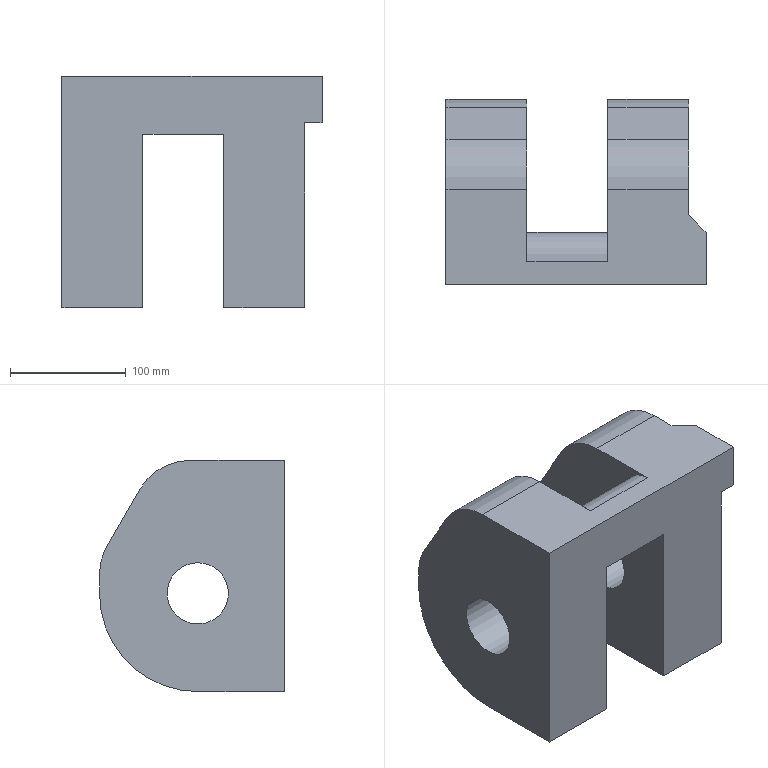Part | NX | features solid 2 | 1 solid | 25 faces | box 225 x 160 x 200 mm | volume 3809518 mm3 | plane 16 | cylinder 9 | commonest cylinder face diameters 100 x4 53 x2 170 x2 50 x1
STEP:
#1=CARTESIAN_POINT('',(925.,625.,111.5));
#2=VERTEX_POINT('',#1);
#3=CARTESIAN_POINT('',(925.,625.,85.));
#4=DIRECTION('',(-1.,0.,0.));
#5=DIRECTION('',(0.,0.,1.));
#6=AXIS2_PLACEMENT_3D('',#3,#4,#5);
#7=CIRCLE('',#6,26.5);
#8=EDGE_CURVE('',#2,#2,#7,.T.);
#9=ORIENTED_EDGE('',*,*,#8,.T.);
#10=EDGE_LOOP('',(#9));
#11=FACE_BOUND('',#10,.T.);
#12=CARTESIAN_POINT('',(995.,625.,111.5));
#13=VERTEX_POINT('',#12);
#14=CARTESIAN_POINT('',(995.,625.,85.));
#15=DIRECTION('',(-1.,0.,0.));
#16=DIRECTION('',(0.,0.,1.));
#17=AXIS2_PLACEMENT_3D('',#14,#15,#16);
#18=CIRCLE('',#17,26.5);
#19=EDGE_CURVE('',#13,#13,#18,.T.);
#20=ORIENTED_EDGE('',*,*,#19,.F.);
#21=EDGE_LOOP('',(#20));
#22=FACE_BOUND('',#21,.T.);
#23=CARTESIAN_POINT('',(915.,625.,85.));
#24=DIRECTION('',(1.,0.,0.));
#25=DIRECTION('',(0.,0.,1.));
#26=AXIS2_PLACEMENT_3D('',#23,#24,#25);
#27=CYLINDRICAL_SURFACE('',#26,26.5);
#28=ADVANCED_FACE('',(#11,#22),#27,.F.);
#29=CARTESIAN_POINT('',(995.,631.906,200.));
#30=VERTEX_POINT('',#29);
#31=CARTESIAN_POINT('',(995.,675.207,175.));
#32=VERTEX_POINT('',#31);
#33=CARTESIAN_POINT('',(995.,631.906,150.));
#34=DIRECTION('',(-1.,0.,0.));
#35=DIRECTION('',(0.,0.,1.));
#36=AXIS2_PLACEMENT_3D('',#33,#34,#35);
#37=CIRCLE('',#36,50.);
#38=EDGE_CURVE('',#30,#32,#37,.T.);
#39=ORIENTED_EDGE('',*,*,#38,.T.);
#40=CARTESIAN_POINT('',(925.,675.207,175.));
#41=VERTEX_POINT('',#40);
#42=CARTESIAN_POINT('',(915.,675.207,175.));
#43=DIRECTION('',(1.,0.,0.));
#44=VECTOR('',#43,1000.);
#45=LINE('',#42,#44);
#46=EDGE_CURVE('',#41,#32,#45,.T.);
#47=ORIENTED_EDGE('',*,*,#46,.F.);
#48=CARTESIAN_POINT('',(925.,631.906,200.));
#49=VERTEX_POINT('',#48);
#50=CARTESIAN_POINT('',(925.,631.906,150.));
#51=DIRECTION('',(-1.,0.,0.));
#52=DIRECTION('',(0.,0.,1.));
#53=AXIS2_PLACEMENT_3D('',#50,#51,#52);
#54=CIRCLE('',#53,50.);
#55=EDGE_CURVE('',#49,#41,#54,.T.);
#56=ORIENTED_EDGE('',*,*,#55,.F.);
#57=CARTESIAN_POINT('',(915.,631.906,200.));
#58=DIRECTION('',(1.,0.,0.));
#59=VECTOR('',#58,1000.);
#60=LINE('',#57,#59);
#61=EDGE_CURVE('',#49,#30,#60,.T.);
#62=ORIENTED_EDGE('',*,*,#61,.T.);
#63=EDGE_LOOP('',(#39,#47,#56,#62));
#64=FACE_BOUND('',#63,.T.);
#65=CARTESIAN_POINT('',(915.,631.906,150.));
#66=DIRECTION('',(1.,0.,0.));
#67=DIRECTION('',(0.,0.,1.));
#68=AXIS2_PLACEMENT_3D('',#65,#66,#67);
#69=CYLINDRICAL_SURFACE('',#68,50.);
#70=ADVANCED_FACE('',(#64),#69,.T.);
#71=CARTESIAN_POINT('',(995.,703.301,126.34));
#72=VERTEX_POINT('',#71);
#73=CARTESIAN_POINT('',(995.,655.,210.));
#74=DIRECTION('',(0.,0.5,-0.866));
#75=VECTOR('',#74,1000.);
#76=LINE('',#73,#75);
#77=EDGE_CURVE('',#32,#72,#76,.T.);
#78=ORIENTED_EDGE('',*,*,#77,.T.);
#79=CARTESIAN_POINT('',(925.,703.301,126.34));
#80=VERTEX_POINT('',#79);
#81=CARTESIAN_POINT('',(915.,703.301,126.34));
#82=DIRECTION('',(1.,0.,0.));
#83=VECTOR('',#82,1000.);
#84=LINE('',#81,#83);
#85=EDGE_CURVE('',#80,#72,#84,.T.);
#86=ORIENTED_EDGE('',*,*,#85,.F.);
#87=CARTESIAN_POINT('',(925.,655.,210.));
#88=DIRECTION('',(0.,0.5,-0.866));
#89=VECTOR('',#88,1000.);
#90=LINE('',#87,#89);
#91=EDGE_CURVE('',#41,#80,#90,.T.);
#92=ORIENTED_EDGE('',*,*,#91,.F.);
#93=ORIENTED_EDGE('',*,*,#46,.T.);
#94=EDGE_LOOP('',(#78,#86,#92,#93));
#95=FACE_BOUND('',#94,.T.);
#96=CARTESIAN_POINT('',(915.,655.,210.));
#97=DIRECTION('',(0.,-0.866,-0.5));
#98=DIRECTION('',(0.,0.5,-0.866));
#99=AXIS2_PLACEMENT_3D('',#96,#97,#98);
#100=PLANE('',#99);
#101=ADVANCED_FACE('',(#95),#100,.F.);
#102=CARTESIAN_POINT('',(995.,710.,101.34));
#103=VERTEX_POINT('',#102);
#104=CARTESIAN_POINT('',(995.,660.,101.34));
#105=DIRECTION('',(-1.,0.,0.));
#106=DIRECTION('',(0.,0.,1.));
#107=AXIS2_PLACEMENT_3D('',#104,#105,#106);
#108=CIRCLE('',#107,50.);
#109=EDGE_CURVE('',#72,#103,#108,.T.);
#110=ORIENTED_EDGE('',*,*,#109,.T.);
#111=CARTESIAN_POINT('',(925.,710.,101.34));
#112=VERTEX_POINT('',#111);
#113=CARTESIAN_POINT('',(915.,710.,101.34));
#114=DIRECTION('',(1.,0.,0.));
#115=VECTOR('',#114,1000.);
#116=LINE('',#113,#115);
#117=EDGE_CURVE('',#112,#103,#116,.T.);
#118=ORIENTED_EDGE('',*,*,#117,.F.);
#119=CARTESIAN_POINT('',(925.,660.,101.34));
#120=DIRECTION('',(-1.,0.,0.));
#121=DIRECTION('',(0.,0.,1.));
#122=AXIS2_PLACEMENT_3D('',#119,#120,#121);
#123=CIRCLE('',#122,50.);
#124=EDGE_CURVE('',#80,#112,#123,.T.);
#125=ORIENTED_EDGE('',*,*,#124,.F.);
#126=ORIENTED_EDGE('',*,*,#85,.T.);
#127=EDGE_LOOP('',(#110,#118,#125,#126));
#128=FACE_BOUND('',#127,.T.);
#129=CARTESIAN_POINT('',(915.,660.,101.34));
#130=DIRECTION('',(1.,0.,0.));
#131=DIRECTION('',(0.,0.,1.));
#132=AXIS2_PLACEMENT_3D('',#129,#130,#131);
#133=CYLINDRICAL_SURFACE('',#132,50.);
#134=ADVANCED_FACE('',(#128),#133,.T.);
#135=CARTESIAN_POINT('',(995.,710.,85.));
#136=VERTEX_POINT('',#135);
#137=CARTESIAN_POINT('',(995.,710.,85.));
#138=DIRECTION('',(0.,0.,1.));
#139=VECTOR('',#138,1000.);
#140=LINE('',#137,#139);
#141=EDGE_CURVE('',#136,#103,#140,.T.);
#142=ORIENTED_EDGE('',*,*,#141,.F.);
#143=CARTESIAN_POINT('',(925.,710.,85.));
#144=VERTEX_POINT('',#143);
#145=CARTESIAN_POINT('',(915.,710.,85.));
#146=DIRECTION('',(1.,0.,0.));
#147=VECTOR('',#146,1000.);
#148=LINE('',#145,#147);
#149=EDGE_CURVE('',#144,#136,#148,.T.);
#150=ORIENTED_EDGE('',*,*,#149,.F.);
#151=CARTESIAN_POINT('',(925.,710.,85.));
#152=DIRECTION('',(0.,0.,1.));
#153=VECTOR('',#152,1000.);
#154=LINE('',#151,#153);
#155=EDGE_CURVE('',#144,#112,#154,.T.);
#156=ORIENTED_EDGE('',*,*,#155,.T.);
#157=ORIENTED_EDGE('',*,*,#117,.T.);
#158=EDGE_LOOP('',(#142,#150,#156,#157));
#159=FACE_BOUND('',#158,.T.);
#160=CARTESIAN_POINT('',(915.,710.,85.));
#161=DIRECTION('',(0.,1.,0.));
#162=DIRECTION('',(0.,0.,1.));
#163=AXIS2_PLACEMENT_3D('',#160,#161,#162);
#164=PLANE('',#163);
#165=ADVANCED_FACE('',(#159),#164,.T.);
#166=CARTESIAN_POINT('',(995.,570.,150.));
#167=VERTEX_POINT('',#166);
#168=CARTESIAN_POINT('',(995.,570.,200.));
#169=VERTEX_POINT('',#168);
#170=CARTESIAN_POINT('',(995.,570.,175.));
#171=DIRECTION('',(1.,0.,0.));
#172=DIRECTION('',(0.,0.,1.));
#173=AXIS2_PLACEMENT_3D('',#170,#171,#172);
#174=CIRCLE('',#173,25.);
#175=EDGE_CURVE('',#167,#169,#174,.T.);
#176=ORIENTED_EDGE('',*,*,#175,.T.);
#177=CARTESIAN_POINT('',(1045.001,570.,200.));
#178=VERTEX_POINT('',#177);
#179=CARTESIAN_POINT('',(975.001,570.,200.));
#180=DIRECTION('',(1.,0.,0.));
#181=VECTOR('',#180,1000.);
#182=LINE('',#179,#181);
#183=EDGE_CURVE('',#169,#178,#182,.T.);
#184=ORIENTED_EDGE('',*,*,#183,.T.);
#185=CARTESIAN_POINT('',(1065.,570.,200.));
#186=VERTEX_POINT('',#185);
#187=CARTESIAN_POINT('',(1055.,570.,200.));
#188=DIRECTION('',(-1.,0.,0.));
#189=VECTOR('',#188,1000.);
#190=LINE('',#187,#189);
#191=EDGE_CURVE('',#178,#186,#190,.F.);
#192=ORIENTED_EDGE('',*,*,#191,.T.);
#193=CARTESIAN_POINT('',(1065.,570.,150.));
#194=VERTEX_POINT('',#193);
#195=CARTESIAN_POINT('',(1065.,570.,175.));
#196=DIRECTION('',(1.,0.,0.));
#197=DIRECTION('',(0.,0.,1.));
#198=AXIS2_PLACEMENT_3D('',#195,#196,#197);
#199=CIRCLE('',#198,25.);
#200=EDGE_CURVE('',#194,#186,#199,.T.);
#201=ORIENTED_EDGE('',*,*,#200,.F.);
#202=CARTESIAN_POINT('',(975.001,570.,150.));
#203=DIRECTION('',(1.,0.,0.));
#204=VECTOR('',#203,1000.);
#205=LINE('',#202,#204);
#206=EDGE_CURVE('',#167,#194,#205,.T.);
#207=ORIENTED_EDGE('',*,*,#206,.F.);
#208=EDGE_LOOP('',(#176,#184,#192,#201,#207));
#209=FACE_BOUND('',#208,.T.);
#210=CARTESIAN_POINT('',(975.001,570.,175.));
#211=DIRECTION('',(1.,0.,0.));
#212=DIRECTION('',(0.,-1.,0.));
#213=AXIS2_PLACEMENT_3D('',#210,#211,#212);
#214=CYLINDRICAL_SURFACE('',#213,25.);
#215=ADVANCED_FACE('',(#209),#214,.T.);
#216=CARTESIAN_POINT('',(1065.,710.,85.));
#217=VERTEX_POINT('',#216);
#218=CARTESIAN_POINT('',(1065.,710.,101.34));
#219=VERTEX_POINT('',#218);
#220=CARTESIAN_POINT('',(1065.,710.,85.));
#221=DIRECTION('',(0.,0.,1.));
#222=VECTOR('',#221,1000.);
#223=LINE('',#220,#222);
#224=EDGE_CURVE('',#217,#219,#223,.T.);
#225=ORIENTED_EDGE('',*,*,#224,.T.);
#226=CARTESIAN_POINT('',(1135.,710.,101.34));
#227=VERTEX_POINT('',#226);
#228=CARTESIAN_POINT('',(1125.,710.,101.34));
#229=DIRECTION('',(1.,0.,0.));
#230=VECTOR('',#229,1000.);
#231=LINE('',#228,#230);
#232=EDGE_CURVE('',#219,#227,#231,.T.);
#233=ORIENTED_EDGE('',*,*,#232,.T.);
#234=CARTESIAN_POINT('',(1135.,710.,85.));
#235=VERTEX_POINT('',#234);
#236=CARTESIAN_POINT('',(1135.,710.,85.));
#237=DIRECTION('',(0.,0.,1.));
#238=VECTOR('',#237,1000.);
#239=LINE('',#236,#238);
#240=EDGE_CURVE('',#235,#227,#239,.T.);
#241=ORIENTED_EDGE('',*,*,#240,.F.);
#242=CARTESIAN_POINT('',(1125.,710.,85.));
#243=DIRECTION('',(-1.,0.,0.));
#244=VECTOR('',#243,1000.);
#245=LINE('',#242,#244);
#246=EDGE_CURVE('',#235,#217,#245,.T.);
#247=ORIENTED_EDGE('',*,*,#246,.T.);
#248=EDGE_LOOP('',(#225,#233,#241,#247));
#249=FACE_BOUND('',#248,.T.);
#250=CARTESIAN_POINT('',(1125.,710.,85.));
#251=DIRECTION('',(0.,-1.,0.));
#252=DIRECTION('',(0.,0.,-1.));
#253=AXIS2_PLACEMENT_3D('',#250,#251,#252);
#254=PLANE('',#253);
#255=ADVANCED_FACE('',(#249),#254,.F.);
#256=CARTESIAN_POINT('',(1135.,703.301,126.34));
#257=VERTEX_POINT('',#256);
#258=CARTESIAN_POINT('',(1135.,660.,101.34));
#259=DIRECTION('',(1.,0.,0.));
#260=DIRECTION('',(0.,1.,0.));
#261=AXIS2_PLACEMENT_3D('',#258,#259,#260);
#262=CIRCLE('',#261,50.);
#263=EDGE_CURVE('',#227,#257,#262,.T.);
#264=ORIENTED_EDGE('',*,*,#263,.F.);
#265=ORIENTED_EDGE('',*,*,#232,.F.);
#266=CARTESIAN_POINT('',(1065.,703.301,126.34));
#267=VERTEX_POINT('',#266);
#268=CARTESIAN_POINT('',(1065.,660.,101.34));
#269=DIRECTION('',(-1.,0.,0.));
#270=DIRECTION('',(0.,0.,1.));
#271=AXIS2_PLACEMENT_3D('',#268,#269,#270);
#272=CIRCLE('',#271,50.);
#273=EDGE_CURVE('',#267,#219,#272,.T.);
#274=ORIENTED_EDGE('',*,*,#273,.F.);
#275=CARTESIAN_POINT('',(1055.,703.301,126.34));
#276=DIRECTION('',(-1.,0.,0.));
#277=VECTOR('',#276,1000.);
#278=LINE('',#275,#277);
#279=EDGE_CURVE('',#257,#267,#278,.T.);
#280=ORIENTED_EDGE('',*,*,#279,.F.);
#281=EDGE_LOOP('',(#264,#265,#274,#280));
#282=FACE_BOUND('',#281,.T.);
#283=CARTESIAN_POINT('',(1125.,660.,101.34));
#284=DIRECTION('',(1.,0.,0.));
#285=DIRECTION('',(0.,0.,1.));
#286=AXIS2_PLACEMENT_3D('',#283,#284,#285);
#287=CYLINDRICAL_SURFACE('',#286,50.);
#288=ADVANCED_FACE('',(#282),#287,.T.);
#289=CARTESIAN_POINT('',(1065.,675.207,175.));
#290=VERTEX_POINT('',#289);
#291=CARTESIAN_POINT('',(1065.,655.,210.));
#292=DIRECTION('',(0.,0.5,-0.866));
#293=VECTOR('',#292,1000.);
#294=LINE('',#291,#293);
#295=EDGE_CURVE('',#290,#267,#294,.T.);
#296=ORIENTED_EDGE('',*,*,#295,.F.);
#297=CARTESIAN_POINT('',(1135.,675.207,175.));
#298=VERTEX_POINT('',#297);
#299=CARTESIAN_POINT('',(1125.,675.207,175.));
#300=DIRECTION('',(1.,0.,0.));
#301=VECTOR('',#300,1000.);
#302=LINE('',#299,#301);
#303=EDGE_CURVE('',#290,#298,#302,.T.);
#304=ORIENTED_EDGE('',*,*,#303,.T.);
#305=CARTESIAN_POINT('',(1135.,655.,210.));
#306=DIRECTION('',(0.,0.5,-0.866));
#307=VECTOR('',#306,1000.);
#308=LINE('',#305,#307);
#309=EDGE_CURVE('',#298,#257,#308,.T.);
#310=ORIENTED_EDGE('',*,*,#309,.T.);
#311=ORIENTED_EDGE('',*,*,#279,.T.);
#312=EDGE_LOOP('',(#296,#304,#310,#311));
#313=FACE_BOUND('',#312,.T.);
#314=CARTESIAN_POINT('',(1125.,655.,210.));
#315=DIRECTION('',(0.,0.866,0.5));
#316=DIRECTION('',(0.,-0.5,0.866));
#317=AXIS2_PLACEMENT_3D('',#314,#315,#316);
#318=PLANE('',#317);
#319=ADVANCED_FACE('',(#313),#318,.T.);
#320=CARTESIAN_POINT('',(1135.,631.906,200.));
#321=VERTEX_POINT('',#320);
#322=CARTESIAN_POINT('',(1135.,631.906,150.));
#323=DIRECTION('',(1.,0.,0.));
#324=DIRECTION('',(0.,1.,0.));
#325=AXIS2_PLACEMENT_3D('',#322,#323,#324);
#326=CIRCLE('',#325,50.);
#327=EDGE_CURVE('',#298,#321,#326,.T.);
#328=ORIENTED_EDGE('',*,*,#327,.F.);
#329=ORIENTED_EDGE('',*,*,#303,.F.);
#330=CARTESIAN_POINT('',(1065.,631.906,200.));
#331=VERTEX_POINT('',#330);
#332=CARTESIAN_POINT('',(1065.,631.906,150.));
#333=DIRECTION('',(-1.,0.,0.));
#334=DIRECTION('',(0.,0.,1.));
#335=AXIS2_PLACEMENT_3D('',#332,#333,#334);
#336=CIRCLE('',#335,50.);
#337=EDGE_CURVE('',#331,#290,#336,.T.);
#338=ORIENTED_EDGE('',*,*,#337,.F.);
#339=CARTESIAN_POINT('',(1145.001,631.906,200.));
#340=DIRECTION('',(-1.,0.,0.));
#341=VECTOR('',#340,1000.);
#342=LINE('',#339,#341);
#343=EDGE_CURVE('',#321,#331,#342,.T.);
#344=ORIENTED_EDGE('',*,*,#343,.F.);
#345=EDGE_LOOP('',(#328,#329,#338,#344));
#346=FACE_BOUND('',#345,.T.);
#347=CARTESIAN_POINT('',(1145.001,631.906,150.));
#348=DIRECTION('',(-1.,0.,0.));
#349=DIRECTION('',(0.,0.,-1.));
#350=AXIS2_PLACEMENT_3D('',#347,#348,#349);
#351=CYLINDRICAL_SURFACE('',#350,50.);
#352=ADVANCED_FACE('',(#346),#351,.T.);
#353=CARTESIAN_POINT('',(1135.,625.,58.5));
#354=VERTEX_POINT('',#353);
#355=CARTESIAN_POINT('',(1135.,625.,85.));
#356=DIRECTION('',(-1.,0.,0.));
#357=DIRECTION('',(0.,0.,-1.));
#358=AXIS2_PLACEMENT_3D('',#355,#356,#357);
#359=CIRCLE('',#358,26.5);
#360=EDGE_CURVE('',#354,#354,#359,.T.);
#361=ORIENTED_EDGE('',*,*,#360,.F.);
#362=EDGE_LOOP('',(#361));
#363=FACE_BOUND('',#362,.T.);
#364=CARTESIAN_POINT('',(1065.,625.,111.5));
#365=VERTEX_POINT('',#364);
#366=CARTESIAN_POINT('',(1065.,625.,85.));
#367=DIRECTION('',(-1.,0.,0.));
#368=DIRECTION('',(0.,0.,1.));
#369=AXIS2_PLACEMENT_3D('',#366,#367,#368);
#370=CIRCLE('',#369,26.5);
#371=EDGE_CURVE('',#365,#365,#370,.T.);
#372=ORIENTED_EDGE('',*,*,#371,.T.);
#373=EDGE_LOOP('',(#372));
#374=FACE_BOUND('',#373,.T.);
#375=CARTESIAN_POINT('',(905.001,625.,85.));
#376=DIRECTION('',(1.,0.,0.));
#377=DIRECTION('',(0.,-1.,0.));
#378=AXIS2_PLACEMENT_3D('',#375,#376,#377);
#379=CYLINDRICAL_SURFACE('',#378,26.5);
#380=ADVANCED_FACE('',(#363,#374),#379,.F.);
#381=CARTESIAN_POINT('',(995.,625.,0.));
#382=VERTEX_POINT('',#381);
#383=CARTESIAN_POINT('',(995.,625.,85.));
#384=DIRECTION('',(1.,0.,0.));
#385=DIRECTION('',(0.,0.,1.));
#386=AXIS2_PLACEMENT_3D('',#383,#384,#385);
#387=CIRCLE('',#386,85.);
#388=EDGE_CURVE('',#382,#136,#387,.T.);
#389=ORIENTED_EDGE('',*,*,#388,.F.);
#390=CARTESIAN_POINT('',(925.,625.,0.));
#391=VERTEX_POINT('',#390);
#392=CARTESIAN_POINT('',(915.,625.,0.));
#393=DIRECTION('',(1.,0.,0.));
#394=VECTOR('',#393,1000.);
#395=LINE('',#392,#394);
#396=EDGE_CURVE('',#391,#382,#395,.T.);
#397=ORIENTED_EDGE('',*,*,#396,.F.);
#398=CARTESIAN_POINT('',(925.,625.,85.));
#399=DIRECTION('',(1.,0.,0.));
#400=DIRECTION('',(0.,0.,1.));
#401=AXIS2_PLACEMENT_3D('',#398,#399,#400);
#402=CIRCLE('',#401,85.);
#403=EDGE_CURVE('',#391,#144,#402,.T.);
#404=ORIENTED_EDGE('',*,*,#403,.T.);
#405=ORIENTED_EDGE('',*,*,#149,.T.);
#406=EDGE_LOOP('',(#389,#397,#404,#405));
#407=FACE_BOUND('',#406,.T.);
#408=CARTESIAN_POINT('',(915.,625.,85.));
#409=DIRECTION('',(1.,0.,0.));
#410=DIRECTION('',(0.,0.,1.));
#411=AXIS2_PLACEMENT_3D('',#408,#409,#410);
#412=CYLINDRICAL_SURFACE('',#411,85.);
#413=ADVANCED_FACE('',(#407),#412,.T.);
#414=CARTESIAN_POINT('',(1065.,625.,0.));
#415=VERTEX_POINT('',#414);
#416=CARTESIAN_POINT('',(1065.,625.,85.));
#417=DIRECTION('',(1.,0.,0.));
#418=DIRECTION('',(0.,0.,1.));
#419=AXIS2_PLACEMENT_3D('',#416,#417,#418);
#420=CIRCLE('',#419,85.);
#421=EDGE_CURVE('',#415,#217,#420,.T.);
#422=ORIENTED_EDGE('',*,*,#421,.T.);
#423=ORIENTED_EDGE('',*,*,#246,.F.);
#424=CARTESIAN_POINT('',(1135.,625.,0.));
#425=VERTEX_POINT('',#424);
#426=CARTESIAN_POINT('',(1135.,625.,85.));
#427=DIRECTION('',(1.,0.,0.));
#428=DIRECTION('',(0.,0.,-1.));
#429=AXIS2_PLACEMENT_3D('',#426,#427,#428);
#430=CIRCLE('',#429,85.);
#431=EDGE_CURVE('',#425,#235,#430,.T.);
#432=ORIENTED_EDGE('',*,*,#431,.F.);
#433=CARTESIAN_POINT('',(1045.001,625.,0.));
#434=DIRECTION('',(1.,0.,0.));
#435=VECTOR('',#434,1000.);
#436=LINE('',#433,#435);
#437=EDGE_CURVE('',#415,#425,#436,.T.);
#438=ORIENTED_EDGE('',*,*,#437,.F.);
#439=EDGE_LOOP('',(#422,#423,#432,#438));
#440=FACE_BOUND('',#439,.T.);
#441=CARTESIAN_POINT('',(1045.001,625.,85.));
#442=DIRECTION('',(1.,0.,0.));
#443=DIRECTION('',(0.,-1.,0.));
#444=AXIS2_PLACEMENT_3D('',#441,#442,#443);
#445=CYLINDRICAL_SURFACE('',#444,85.);
#446=ADVANCED_FACE('',(#440),#445,.T.);
#447=CARTESIAN_POINT('',(995.,550.,150.));
#448=VERTEX_POINT('',#447);
#449=CARTESIAN_POINT('',(995.,710.,150.));
#450=DIRECTION('',(0.,1.,0.));
#451=VECTOR('',#450,1000.);
#452=LINE('',#449,#451);
#453=EDGE_CURVE('',#448,#167,#452,.T.);
#454=ORIENTED_EDGE('',*,*,#453,.T.);
#455=ORIENTED_EDGE('',*,*,#206,.T.);
#456=CARTESIAN_POINT('',(1065.,550.,150.));
#457=VERTEX_POINT('',#456);
#458=CARTESIAN_POINT('',(1065.,710.,150.));
#459=DIRECTION('',(0.,1.,0.));
#460=VECTOR('',#459,1000.);
#461=LINE('',#458,#460);
#462=EDGE_CURVE('',#457,#194,#461,.T.);
#463=ORIENTED_EDGE('',*,*,#462,.F.);
#464=CARTESIAN_POINT('',(975.001,550.,150.));
#465=DIRECTION('',(1.,0.,0.));
#466=VECTOR('',#465,1000.);
#467=LINE('',#464,#466);
#468=EDGE_CURVE('',#448,#457,#467,.T.);
#469=ORIENTED_EDGE('',*,*,#468,.F.);
#470=EDGE_LOOP('',(#454,#455,#463,#469));
#471=FACE_BOUND('',#470,.T.);
#472=CARTESIAN_POINT('',(975.001,550.,150.));
#473=DIRECTION('',(0.,0.,1.));
#474=DIRECTION('',(0.,1.,0.));
#475=AXIS2_PLACEMENT_3D('',#472,#473,#474);
#476=PLANE('',#475);
#477=ADVANCED_FACE('',(#471),#476,.F.);
#478=CARTESIAN_POINT('',(1065.,550.,0.));
#479=VERTEX_POINT('',#478);
#480=CARTESIAN_POINT('',(1065.,710.,0.));
#481=DIRECTION('',(0.,1.,0.));
#482=VECTOR('',#481,1000.);
#483=LINE('',#480,#482);
#484=EDGE_CURVE('',#479,#415,#483,.T.);
#485=ORIENTED_EDGE('',*,*,#484,.T.);
#486=ORIENTED_EDGE('',*,*,#437,.T.);
#487=CARTESIAN_POINT('',(1135.,550.,0.));
#488=VERTEX_POINT('',#487);
#489=CARTESIAN_POINT('',(1135.,70.,0.));
#490=DIRECTION('',(0.,1.,0.));
#491=VECTOR('',#490,1000.);
#492=LINE('',#489,#491);
#493=EDGE_CURVE('',#488,#425,#492,.T.);
#494=ORIENTED_EDGE('',*,*,#493,.F.);
#495=CARTESIAN_POINT('',(401.001,550.,0.));
#496=DIRECTION('',(1.,0.,0.));
#497=VECTOR('',#496,1000.);
#498=LINE('',#495,#497);
#499=EDGE_CURVE('',#479,#488,#498,.T.);
#500=ORIENTED_EDGE('',*,*,#499,.F.);
#501=EDGE_LOOP('',(#485,#486,#494,#500));
#502=FACE_BOUND('',#501,.T.);
#503=CARTESIAN_POINT('',(401.001,70.,0.));
#504=DIRECTION('',(0.,0.,1.));
#505=DIRECTION('',(1.,0.,0.));
#506=AXIS2_PLACEMENT_3D('',#503,#504,#505);
#507=PLANE('',#506);
#508=ADVANCED_FACE('',(#502),#507,.F.);
#509=ORIENTED_EDGE('',*,*,#360,.T.);
#510=EDGE_LOOP('',(#509));
#511=FACE_BOUND('',#510,.T.);
#512=CARTESIAN_POINT('',(1135.,550.,160.));
#513=VERTEX_POINT('',#512);
#514=CARTESIAN_POINT('',(1135.,550.,20.));
#515=DIRECTION('',(0.,0.,1.));
#516=VECTOR('',#515,1000.);
#517=LINE('',#514,#516);
#518=EDGE_CURVE('',#488,#513,#517,.T.);
#519=ORIENTED_EDGE('',*,*,#518,.F.);
#520=ORIENTED_EDGE('',*,*,#493,.T.);
#521=ORIENTED_EDGE('',*,*,#431,.T.);
#522=ORIENTED_EDGE('',*,*,#240,.T.);
#523=ORIENTED_EDGE('',*,*,#263,.T.);
#524=ORIENTED_EDGE('',*,*,#309,.F.);
#525=ORIENTED_EDGE('',*,*,#327,.T.);
#526=CARTESIAN_POINT('',(1135.,610.,200.));
#527=VERTEX_POINT('',#526);
#528=CARTESIAN_POINT('',(1135.,371.797,200.));
#529=DIRECTION('',(0.,-1.,0.));
#530=VECTOR('',#529,1000.);
#531=LINE('',#528,#530);
#532=EDGE_CURVE('',#321,#527,#531,.T.);
#533=ORIENTED_EDGE('',*,*,#532,.T.);
#534=CARTESIAN_POINT('',(1135.,610.,160.));
#535=VERTEX_POINT('',#534);
#536=CARTESIAN_POINT('',(1135.,610.,200.));
#537=DIRECTION('',(0.,0.,-1.));
#538=VECTOR('',#537,1000.);
#539=LINE('',#536,#538);
#540=EDGE_CURVE('',#527,#535,#539,.T.);
#541=ORIENTED_EDGE('',*,*,#540,.T.);
#542=CARTESIAN_POINT('',(1135.,580.,160.));
#543=DIRECTION('',(0.,1.,0.));
#544=VECTOR('',#543,1000.);
#545=LINE('',#542,#544);
#546=EDGE_CURVE('',#513,#535,#545,.T.);
#547=ORIENTED_EDGE('',*,*,#546,.F.);
#548=EDGE_LOOP('',(#519,#520,#521,#522,#523,#524,#525,#533,#541,#547));
#549=FACE_BOUND('',#548,.T.);
#550=CARTESIAN_POINT('',(1135.,371.797,20.));
#551=DIRECTION('',(-1.,0.,0.));
#552=DIRECTION('',(0.,0.,-1.));
#553=AXIS2_PLACEMENT_3D('',#550,#551,#552);
#554=PLANE('',#553);
#555=ADVANCED_FACE('',(#511,#549),#554,.F.);
#556=ORIENTED_EDGE('',*,*,#371,.F.);
#557=EDGE_LOOP('',(#556));
#558=FACE_BOUND('',#557,.T.);
#559=CARTESIAN_POINT('',(1065.,550.,200.));
#560=DIRECTION('',(0.,0.,1.));
#561=VECTOR('',#560,1000.);
#562=LINE('',#559,#561);
#563=EDGE_CURVE('',#479,#457,#562,.T.);
#564=ORIENTED_EDGE('',*,*,#563,.T.);
#565=ORIENTED_EDGE('',*,*,#462,.T.);
#566=ORIENTED_EDGE('',*,*,#200,.T.);
#567=CARTESIAN_POINT('',(1065.,-240.,200.));
#568=DIRECTION('',(0.,-1.,0.));
#569=VECTOR('',#568,1000.);
#570=LINE('',#567,#569);
#571=EDGE_CURVE('',#331,#186,#570,.T.);
#572=ORIENTED_EDGE('',*,*,#571,.F.);
#573=ORIENTED_EDGE('',*,*,#337,.T.);
#574=ORIENTED_EDGE('',*,*,#295,.T.);
#575=ORIENTED_EDGE('',*,*,#273,.T.);
#576=ORIENTED_EDGE('',*,*,#224,.F.);
#577=ORIENTED_EDGE('',*,*,#421,.F.);
#578=ORIENTED_EDGE('',*,*,#484,.F.);
#579=EDGE_LOOP('',(#564,#565,#566,#572,#573,#574,#575,#576,#577,#578));
#580=FACE_BOUND('',#579,.T.);
#581=CARTESIAN_POINT('',(1065.,710.,200.));
#582=DIRECTION('',(-1.,0.,0.));
#583=DIRECTION('',(0.,0.,-1.));
#584=AXIS2_PLACEMENT_3D('',#581,#582,#583);
#585=PLANE('',#584);
#586=ADVANCED_FACE('',(#558,#580),#585,.T.);
#587=CARTESIAN_POINT('',(925.,550.,0.));
#588=VERTEX_POINT('',#587);
#589=CARTESIAN_POINT('',(925.,710.,0.));
#590=DIRECTION('',(0.,1.,0.));
#591=VECTOR('',#590,1000.);
#592=LINE('',#589,#591);
#593=EDGE_CURVE('',#588,#391,#592,.T.);
#594=ORIENTED_EDGE('',*,*,#593,.T.);
#595=ORIENTED_EDGE('',*,*,#396,.T.);
#596=CARTESIAN_POINT('',(995.,550.,0.));
#597=VERTEX_POINT('',#596);
#598=CARTESIAN_POINT('',(995.,710.,0.));
#599=DIRECTION('',(0.,1.,0.));
#600=VECTOR('',#599,1000.);
#601=LINE('',#598,#600);
#602=EDGE_CURVE('',#597,#382,#601,.T.);
#603=ORIENTED_EDGE('',*,*,#602,.F.);
#604=CARTESIAN_POINT('',(401.001,550.,0.));
#605=DIRECTION('',(1.,0.,0.));
#606=VECTOR('',#605,1000.);
#607=LINE('',#604,#606);
#608=EDGE_CURVE('',#588,#597,#607,.T.);
#609=ORIENTED_EDGE('',*,*,#608,.F.);
#610=EDGE_LOOP('',(#594,#595,#603,#609));
#611=FACE_BOUND('',#610,.T.);
#612=CARTESIAN_POINT('',(401.001,70.,0.));
#613=DIRECTION('',(0.,0.,1.));
#614=DIRECTION('',(1.,0.,0.));
#615=AXIS2_PLACEMENT_3D('',#612,#613,#614);
#616=PLANE('',#615);
#617=ADVANCED_FACE('',(#611),#616,.F.);
#618=CARTESIAN_POINT('',(925.,550.,200.));
#619=VERTEX_POINT('',#618);
#620=CARTESIAN_POINT('',(925.,-305.,200.));
#621=DIRECTION('',(0.,1.,0.));
#622=VECTOR('',#621,1000.);
#623=LINE('',#620,#622);
#624=EDGE_CURVE('',#619,#49,#623,.T.);
#625=ORIENTED_EDGE('',*,*,#624,.T.);
#626=ORIENTED_EDGE('',*,*,#55,.T.);
#627=ORIENTED_EDGE('',*,*,#91,.T.);
#628=ORIENTED_EDGE('',*,*,#124,.T.);
#629=ORIENTED_EDGE('',*,*,#155,.F.);
#630=ORIENTED_EDGE('',*,*,#403,.F.);
#631=ORIENTED_EDGE('',*,*,#593,.F.);
#632=CARTESIAN_POINT('',(925.,550.,10.));
#633=DIRECTION('',(0.,0.,-1.));
#634=VECTOR('',#633,1000.);
#635=LINE('',#632,#634);
#636=EDGE_CURVE('',#619,#588,#635,.T.);
#637=ORIENTED_EDGE('',*,*,#636,.F.);
#638=EDGE_LOOP('',(#625,#626,#627,#628,#629,#630,#631,#637));
#639=FACE_BOUND('',#638,.T.);
#640=ORIENTED_EDGE('',*,*,#8,.F.);
#641=EDGE_LOOP('',(#640));
#642=FACE_BOUND('',#641,.T.);
#643=CARTESIAN_POINT('',(925.,-305.,10.));
#644=DIRECTION('',(1.,0.,0.));
#645=DIRECTION('',(0.,0.,-1.));
#646=AXIS2_PLACEMENT_3D('',#643,#644,#645);
#647=PLANE('',#646);
#648=ADVANCED_FACE('',(#639,#642),#647,.F.);
#649=ORIENTED_EDGE('',*,*,#19,.T.);
#650=EDGE_LOOP('',(#649));
#651=FACE_BOUND('',#650,.T.);
#652=ORIENTED_EDGE('',*,*,#602,.T.);
#653=ORIENTED_EDGE('',*,*,#388,.T.);
#654=ORIENTED_EDGE('',*,*,#141,.T.);
#655=ORIENTED_EDGE('',*,*,#109,.F.);
#656=ORIENTED_EDGE('',*,*,#77,.F.);
#657=ORIENTED_EDGE('',*,*,#38,.F.);
#658=CARTESIAN_POINT('',(995.,-240.,200.));
#659=DIRECTION('',(0.,-1.,0.));
#660=VECTOR('',#659,1000.);
#661=LINE('',#658,#660);
#662=EDGE_CURVE('',#30,#169,#661,.T.);
#663=ORIENTED_EDGE('',*,*,#662,.T.);
#664=ORIENTED_EDGE('',*,*,#175,.F.);
#665=ORIENTED_EDGE('',*,*,#453,.F.);
#666=CARTESIAN_POINT('',(995.,550.,200.));
#667=DIRECTION('',(0.,0.,1.));
#668=VECTOR('',#667,1000.);
#669=LINE('',#666,#668);
#670=EDGE_CURVE('',#597,#448,#669,.T.);
#671=ORIENTED_EDGE('',*,*,#670,.F.);
#672=EDGE_LOOP('',(#652,#653,#654,#655,#656,#657,#663,#664,#665,#671));
#673=FACE_BOUND('',#672,.T.);
#674=CARTESIAN_POINT('',(995.,710.,200.));
#675=DIRECTION('',(-1.,0.,0.));
#676=DIRECTION('',(0.,0.,-1.));
#677=AXIS2_PLACEMENT_3D('',#674,#675,#676);
#678=PLANE('',#677);
#679=ADVANCED_FACE('',(#651,#673),#678,.F.);
#680=ORIENTED_EDGE('',*,*,#624,.F.);
#681=CARTESIAN_POINT('',(1150.,550.,200.));
#682=VERTEX_POINT('',#681);
#683=CARTESIAN_POINT('',(-855.,550.,200.));
#684=DIRECTION('',(-1.,0.,0.));
#685=VECTOR('',#684,1000.);
#686=LINE('',#683,#685);
#687=EDGE_CURVE('',#682,#619,#686,.T.);
#688=ORIENTED_EDGE('',*,*,#687,.F.);
#689=CARTESIAN_POINT('',(1150.,595.,200.));
#690=VERTEX_POINT('',#689);
#691=CARTESIAN_POINT('',(1150.,580.,200.));
#692=DIRECTION('',(0.,1.,0.));
#693=VECTOR('',#692,1000.);
#694=LINE('',#691,#693);
#695=EDGE_CURVE('',#682,#690,#694,.T.);
#696=ORIENTED_EDGE('',*,*,#695,.T.);
#697=CARTESIAN_POINT('',(1153.75,591.25,200.));
#698=DIRECTION('',(0.7071,-0.7071,0.));
#699=VECTOR('',#698,1000.);
#700=LINE('',#697,#699);
#701=EDGE_CURVE('',#527,#690,#700,.T.);
#702=ORIENTED_EDGE('',*,*,#701,.F.);
#703=ORIENTED_EDGE('',*,*,#532,.F.);
#704=ORIENTED_EDGE('',*,*,#343,.T.);
#705=ORIENTED_EDGE('',*,*,#571,.T.);
#706=ORIENTED_EDGE('',*,*,#191,.F.);
#707=ORIENTED_EDGE('',*,*,#183,.F.);
#708=ORIENTED_EDGE('',*,*,#662,.F.);
#709=ORIENTED_EDGE('',*,*,#61,.F.);
#710=EDGE_LOOP('',(#680,#688,#696,#702,#703,#704,#705,#706,#707,#708,#709));
#711=FACE_BOUND('',#710,.T.);
#712=CARTESIAN_POINT('',(-855.,115.,200.));
#713=DIRECTION('',(0.,0.,-1.));
#714=DIRECTION('',(0.,-1.,0.));
#715=AXIS2_PLACEMENT_3D('',#712,#713,#714);
#716=PLANE('',#715);
#717=ADVANCED_FACE('',(#711),#716,.F.);
#718=ORIENTED_EDGE('',*,*,#687,.T.);
#719=ORIENTED_EDGE('',*,*,#636,.T.);
#720=ORIENTED_EDGE('',*,*,#608,.T.);
#721=ORIENTED_EDGE('',*,*,#670,.T.);
#722=ORIENTED_EDGE('',*,*,#468,.T.);
#723=ORIENTED_EDGE('',*,*,#563,.F.);
#724=ORIENTED_EDGE('',*,*,#499,.T.);
#725=ORIENTED_EDGE('',*,*,#518,.T.);
#726=CARTESIAN_POINT('',(1150.,550.,160.));
#727=VERTEX_POINT('',#726);
#728=CARTESIAN_POINT('',(1142.5,550.,160.));
#729=DIRECTION('',(-1.,0.,0.));
#730=VECTOR('',#729,1000.);
#731=LINE('',#728,#730);
#732=EDGE_CURVE('',#727,#513,#731,.T.);
#733=ORIENTED_EDGE('',*,*,#732,.F.);
#734=CARTESIAN_POINT('',(1150.,550.,200.));
#735=DIRECTION('',(0.,0.,-1.));
#736=VECTOR('',#735,1000.);
#737=LINE('',#734,#736);
#738=EDGE_CURVE('',#682,#727,#737,.T.);
#739=ORIENTED_EDGE('',*,*,#738,.F.);
#740=EDGE_LOOP('',(#718,#719,#720,#721,#722,#723,#724,#725,#733,#739));
#741=FACE_BOUND('',#740,.T.);
#742=CARTESIAN_POINT('',(-970.,550.,-30.));
#743=DIRECTION('',(0.,1.,0.));
#744=DIRECTION('',(0.,0.,-1.));
#745=AXIS2_PLACEMENT_3D('',#742,#743,#744);
#746=PLANE('',#745);
#747=ADVANCED_FACE('',(#741),#746,.F.);
#748=CARTESIAN_POINT('',(1150.,595.,160.));
#749=VERTEX_POINT('',#748);
#750=CARTESIAN_POINT('',(1150.,580.,160.));
#751=DIRECTION('',(0.,-1.,0.));
#752=VECTOR('',#751,1000.);
#753=LINE('',#750,#752);
#754=EDGE_CURVE('',#749,#727,#753,.T.);
#755=ORIENTED_EDGE('',*,*,#754,.T.);
#756=ORIENTED_EDGE('',*,*,#732,.T.);
#757=ORIENTED_EDGE('',*,*,#546,.T.);
#758=CARTESIAN_POINT('',(1153.75,591.25,160.));
#759=DIRECTION('',(-0.7071,0.7071,0.));
#760=VECTOR('',#759,1000.);
#761=LINE('',#758,#760);
#762=EDGE_CURVE('',#749,#535,#761,.T.);
#763=ORIENTED_EDGE('',*,*,#762,.F.);
#764=EDGE_LOOP('',(#755,#756,#757,#763));
#765=FACE_BOUND('',#764,.T.);
#766=CARTESIAN_POINT('',(1142.5,580.,160.));
#767=DIRECTION('',(0.,0.,-1.));
#768=DIRECTION('',(1.,0.,0.));
#769=AXIS2_PLACEMENT_3D('',#766,#767,#768);
#770=PLANE('',#769);
#771=ADVANCED_FACE('',(#765),#770,.T.);
#772=ORIENTED_EDGE('',*,*,#695,.F.);
#773=ORIENTED_EDGE('',*,*,#738,.T.);
#774=ORIENTED_EDGE('',*,*,#754,.F.);
#775=CARTESIAN_POINT('',(1150.,595.,200.));
#776=DIRECTION('',(0.,0.,-1.));
#777=VECTOR('',#776,1000.);
#778=LINE('',#775,#777);
#779=EDGE_CURVE('',#690,#749,#778,.T.);
#780=ORIENTED_EDGE('',*,*,#779,.F.);
#781=EDGE_LOOP('',(#772,#773,#774,#780));
#782=FACE_BOUND('',#781,.T.);
#783=CARTESIAN_POINT('',(1150.,580.,200.));
#784=DIRECTION('',(1.,0.,0.));
#785=DIRECTION('',(0.,0.,1.));
#786=AXIS2_PLACEMENT_3D('',#783,#784,#785);
#787=PLANE('',#786);
#788=ADVANCED_FACE('',(#782),#787,.T.);
#789=ORIENTED_EDGE('',*,*,#701,.T.);
#790=ORIENTED_EDGE('',*,*,#779,.T.);
#791=ORIENTED_EDGE('',*,*,#762,.T.);
#792=ORIENTED_EDGE('',*,*,#540,.F.);
#793=EDGE_LOOP('',(#789,#790,#791,#792));
#794=FACE_BOUND('',#793,.T.);
#795=CARTESIAN_POINT('',(1150.,595.,200.));
#796=DIRECTION('',(-0.7071,-0.7071,0.));
#797=DIRECTION('',(-0.7071,0.7071,0.));
#798=AXIS2_PLACEMENT_3D('',#795,#796,#797);
#799=PLANE('',#798);
#800=ADVANCED_FACE('',(#794),#799,.F.);
#801=CLOSED_SHELL('',(#28,#70,#101,#134,#165,#215,#255,#288,#319,#352,#380,#413,#446,#477,#508,#555,#586,#617,#648,#679,#717,#747,#771,#788,#800));
#802=MANIFOLD_SOLID_BREP('',#801);
#803=(LENGTH_UNIT()NAMED_UNIT(*)SI_UNIT(.MILLI.,.METRE.));
#804=UNCERTAINTY_MEASURE_WITH_UNIT(LENGTH_MEASURE(0.00001),#803,'','');
#805=(NAMED_UNIT(*)PLANE_ANGLE_UNIT()SI_UNIT($,.RADIAN.));
#806=(NAMED_UNIT(*)SI_UNIT($,.STERADIAN.)SOLID_ANGLE_UNIT());
#807=(GEOMETRIC_REPRESENTATION_CONTEXT(3)GLOBAL_UNCERTAINTY_ASSIGNED_CONTEXT((#804))GLOBAL_UNIT_ASSIGNED_CONTEXT((#803,#805,#806))REPRESENTATION_CONTEXT('',''));
#808=ADVANCED_BREP_SHAPE_REPRESENTATION('',(#802),#807);